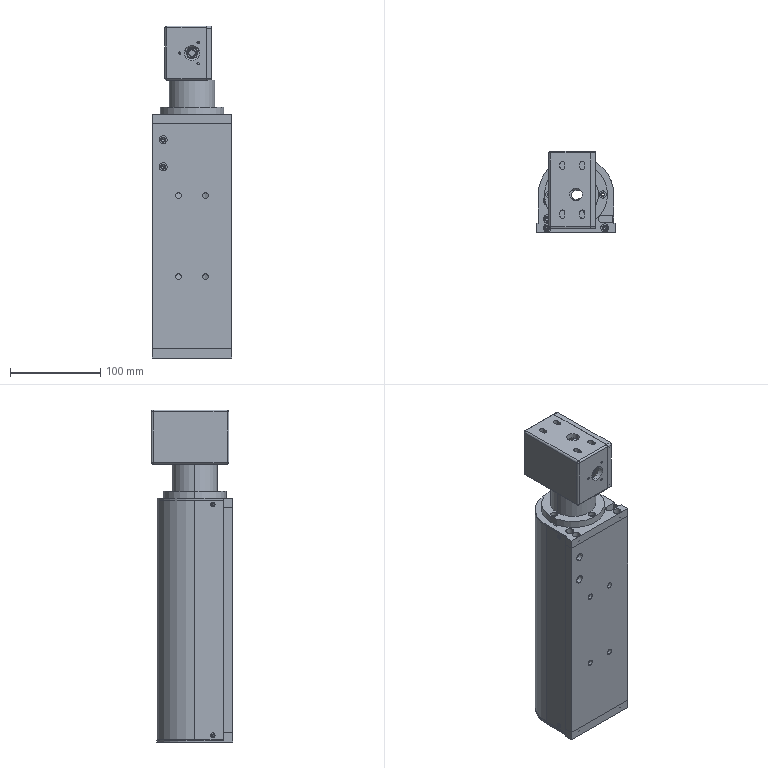Part | SolidWorks | features CompositeCurve 4 | 11 solids | 458 faces | box 88 x 90 x 368 mm | volume 672845 mm3 | cylinder 254 | plane 150 | cone 50 | sphere 4 | commonest cylinder face diameters 4.2 x26 2.5 x24 3.3 x24 5.5 x24 3.5 x18 9 x16